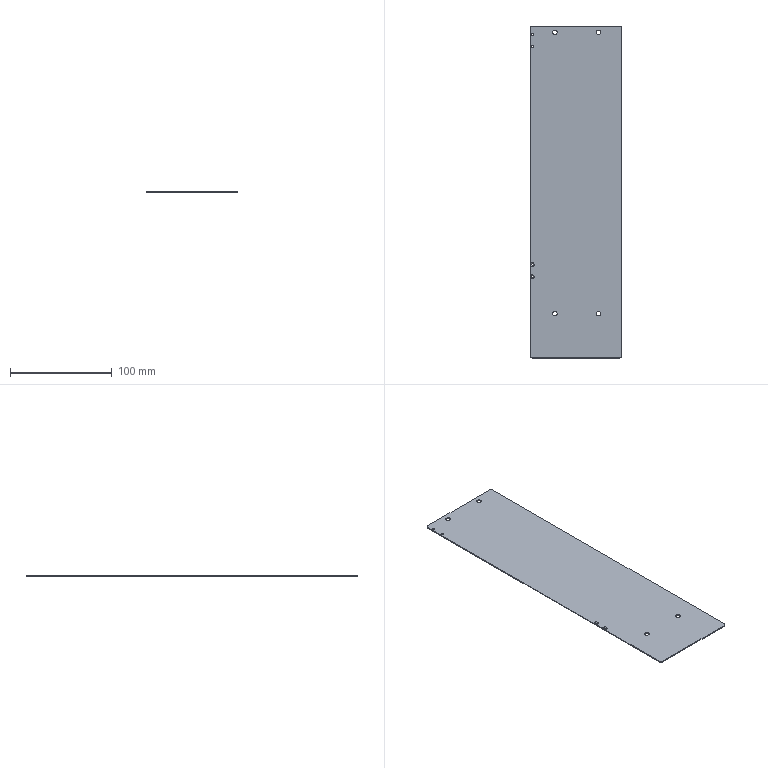Part | STEP file | Combiner mounting plate | 1 solid | 20 faces | box 90 x 325.8 x 1 mm | volume 29233 mm3 | cylinder 12 | plane 6 | cone 2 | commonest cylinder face diameters 2.2 x4 4 x4 4.5 x4